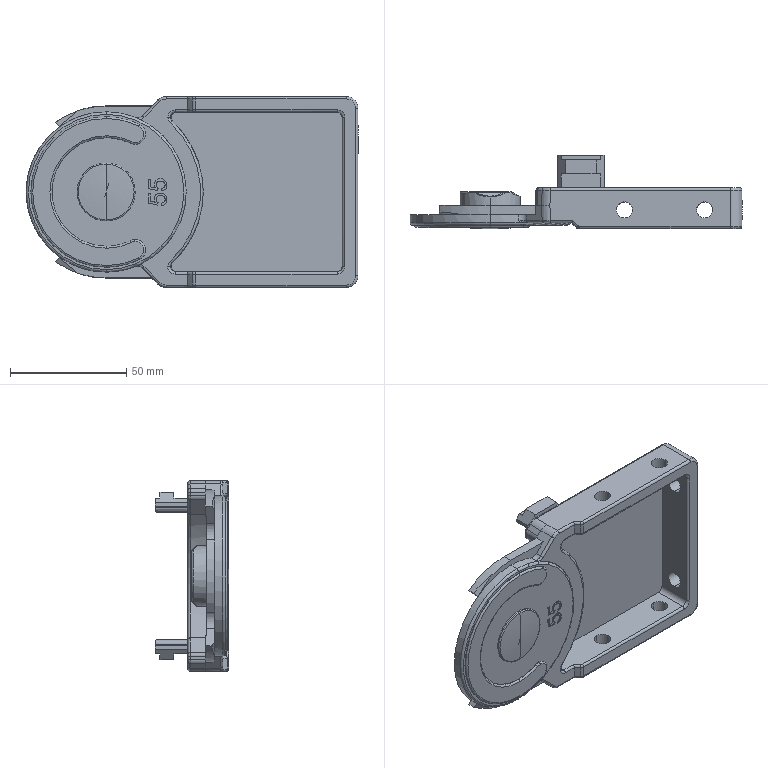Part | SolidWorks | features ICE 3, BaseBody 1 | 1 solid | 383 faces | box 142.639 x 31.5 x 82 mm | volume 72646 mm3 | plane 136 | cone 97 | cylinder 85 | torus 36 | spline 23 | sphere 6 | commonest cylinder face diameters 2 x25 7 x12 4.4 x6 10 x6 5 x4 10.4 x4